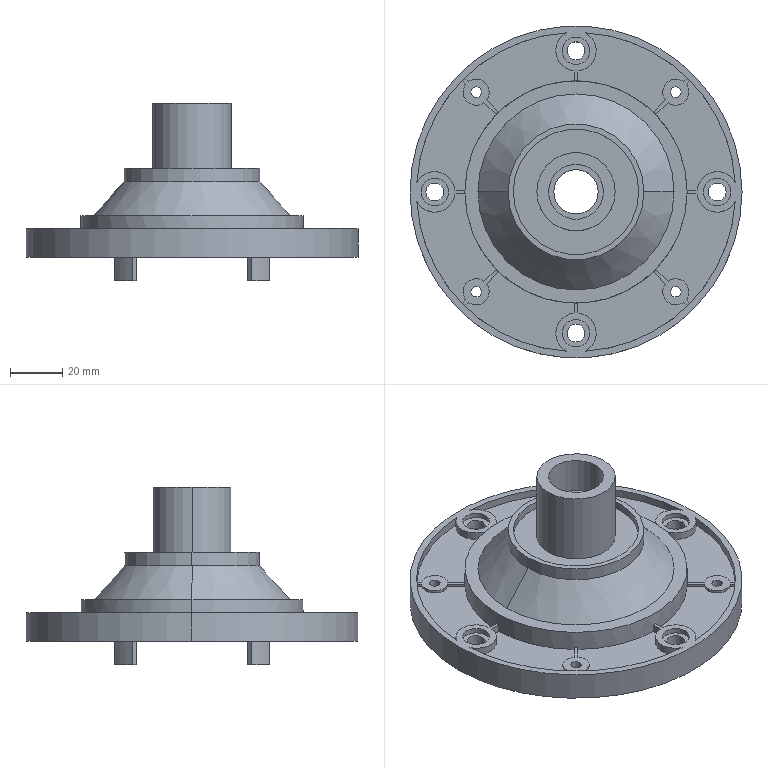Part | SolidWorks | features ICE 14, CirPattern 4, Extrusion 1, RevCut 1, Revolution 1 | 1 solid | 226 faces | box 127 x 127 x 68 mm | volume 67488 mm3 | plane 134 | cylinder 82 | cone 10 | commonest cylinder face diameters 10.5 x16 10 x12 15.5 x10 4 x8 6.8 x8 122 x4